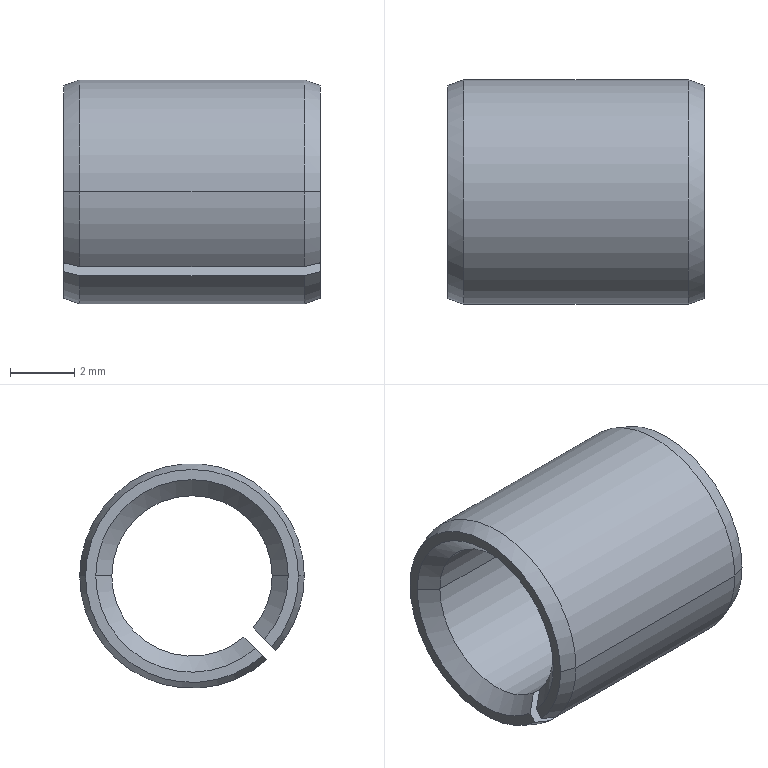Part | NX | 1 solid | 22 faces | box 8 x 7 x 7 mm | volume 141.575 mm3 | cone 12 | cylinder 6 | plane 4 | commonest cylinder face diameters 5 x3 7 x3
STEP:
#1=CARTESIAN_POINT('',(0.5,-2.5,0.));
#2=VERTEX_POINT('',#1);
#3=CARTESIAN_POINT('',(0.,-3.,0.));
#4=VERTEX_POINT('',#3);
#5=CARTESIAN_POINT('',(0.25,-2.75,0.));
#6=DIRECTION('',(-0.7071,-0.7071,0.));
#7=VECTOR('',#6,1000.);
#8=LINE('',#5,#7);
#9=EDGE_CURVE('',#2,#4,#8,.T.);
#10=ORIENTED_EDGE('',*,*,#9,.F.);
#11=CARTESIAN_POINT('',(0.5,-1.904,-1.621));
#12=VERTEX_POINT('',#11);
#13=CARTESIAN_POINT('',(0.5,0.,0.));
#14=DIRECTION('',(-1.,0.,0.));
#15=DIRECTION('',(0.,1.,0.));
#16=AXIS2_PLACEMENT_3D('',#13,#14,#15);
#17=CIRCLE('',#16,2.5);
#18=EDGE_CURVE('',#12,#2,#17,.T.);
#19=ORIENTED_EDGE('',*,*,#18,.F.);
#20=CARTESIAN_POINT('',(0.,-2.258,-1.975));
#21=VERTEX_POINT('',#20);
#22=CARTESIAN_POINT('',(0.5,-1.904,-1.621));
#23=CARTESIAN_POINT('',(0.2728,-2.065,-1.782));
#24=CARTESIAN_POINT('',(0.,-2.258,-1.975));
#25=(BOUNDED_CURVE()B_SPLINE_CURVE(2,(#22,#23,#24),.UNSPECIFIED.,.F.,.F.)B_SPLINE_CURVE_WITH_KNOTS((3,3),(0.,0.7081),.UNSPECIFIED.)CURVE()GEOMETRIC_REPRESENTATION_ITEM()RATIONAL_B_SPLINE_CURVE((1.,1.004,1.))REPRESENTATION_ITEM(''));
#26=EDGE_CURVE('',#12,#21,#25,.T.);
#27=ORIENTED_EDGE('',*,*,#26,.T.);
#28=CARTESIAN_POINT('',(0.,0.,0.));
#29=DIRECTION('',(-1.,0.,0.));
#30=DIRECTION('',(0.,1.,0.));
#31=AXIS2_PLACEMENT_3D('',#28,#29,#30);
#32=CIRCLE('',#31,3.);
#33=EDGE_CURVE('',#21,#4,#32,.T.);
#34=ORIENTED_EDGE('',*,*,#33,.T.);
#35=EDGE_LOOP('',(#10,#19,#27,#34));
#36=FACE_BOUND('',#35,.T.);
#37=CARTESIAN_POINT('',(0.25,0.,0.));
#38=DIRECTION('',(-1.,0.,0.));
#39=DIRECTION('',(0.,1.,0.));
#40=AXIS2_PLACEMENT_3D('',#37,#38,#39);
#41=CONICAL_SURFACE('',#40,2.75,0.7854);
#42=ADVANCED_FACE('',(#36),#41,.F.);
#43=CARTESIAN_POINT('',(8.,-1.975,-2.258));
#44=VERTEX_POINT('',#43);
#45=CARTESIAN_POINT('',(8.,-2.201,-2.483));
#46=VERTEX_POINT('',#45);
#47=CARTESIAN_POINT('',(8.,0.9312,0.6483));
#48=DIRECTION('',(0.,-0.7071,-0.7071));
#49=VECTOR('',#48,1000.);
#50=LINE('',#47,#49);
#51=EDGE_CURVE('',#44,#46,#50,.T.);
#52=ORIENTED_EDGE('',*,*,#51,.T.);
#53=CARTESIAN_POINT('',(8.,3.318,0.));
#54=VERTEX_POINT('',#53);
#55=CARTESIAN_POINT('',(8.,0.,0.));
#56=DIRECTION('',(-1.,0.,0.));
#57=DIRECTION('',(0.,1.,0.));
#58=AXIS2_PLACEMENT_3D('',#55,#56,#57);
#59=CIRCLE('',#58,3.318);
#60=EDGE_CURVE('',#54,#46,#59,.T.);
#61=ORIENTED_EDGE('',*,*,#60,.F.);
#62=CARTESIAN_POINT('',(8.,-3.318,0.));
#63=VERTEX_POINT('',#62);
#64=CARTESIAN_POINT('',(8.,0.,0.));
#65=DIRECTION('',(-1.,0.,0.));
#66=DIRECTION('',(0.,1.,0.));
#67=AXIS2_PLACEMENT_3D('',#64,#65,#66);
#68=CIRCLE('',#67,3.318);
#69=EDGE_CURVE('',#63,#54,#68,.T.);
#70=ORIENTED_EDGE('',*,*,#69,.F.);
#71=CARTESIAN_POINT('',(8.,-2.483,-2.201));
#72=VERTEX_POINT('',#71);
#73=CARTESIAN_POINT('',(8.,0.,0.));
#74=DIRECTION('',(-1.,0.,0.));
#75=DIRECTION('',(0.,1.,0.));
#76=AXIS2_PLACEMENT_3D('',#73,#74,#75);
#77=CIRCLE('',#76,3.318);
#78=EDGE_CURVE('',#72,#63,#77,.T.);
#79=ORIENTED_EDGE('',*,*,#78,.F.);
#80=CARTESIAN_POINT('',(8.,-2.258,-1.975));
#81=VERTEX_POINT('',#80);
#82=CARTESIAN_POINT('',(8.,-1.827,-1.544));
#83=DIRECTION('',(0.,0.7071,0.7071));
#84=VECTOR('',#83,1000.);
#85=LINE('',#82,#84);
#86=EDGE_CURVE('',#72,#81,#85,.T.);
#87=ORIENTED_EDGE('',*,*,#86,.T.);
#88=CARTESIAN_POINT('',(8.,-3.,0.));
#89=VERTEX_POINT('',#88);
#90=CARTESIAN_POINT('',(8.,0.,0.));
#91=DIRECTION('',(-1.,0.,0.));
#92=DIRECTION('',(0.,1.,0.));
#93=AXIS2_PLACEMENT_3D('',#90,#91,#92);
#94=CIRCLE('',#93,3.);
#95=EDGE_CURVE('',#81,#89,#94,.T.);
#96=ORIENTED_EDGE('',*,*,#95,.T.);
#97=CARTESIAN_POINT('',(8.,3.,0.));
#98=VERTEX_POINT('',#97);
#99=CARTESIAN_POINT('',(8.,0.,0.));
#100=DIRECTION('',(-1.,0.,0.));
#101=DIRECTION('',(0.,1.,0.));
#102=AXIS2_PLACEMENT_3D('',#99,#100,#101);
#103=CIRCLE('',#102,3.);
#104=EDGE_CURVE('',#89,#98,#103,.T.);
#105=ORIENTED_EDGE('',*,*,#104,.T.);
#106=CARTESIAN_POINT('',(8.,0.,0.));
#107=DIRECTION('',(-1.,0.,0.));
#108=DIRECTION('',(0.,1.,0.));
#109=AXIS2_PLACEMENT_3D('',#106,#107,#108);
#110=CIRCLE('',#109,3.);
#111=EDGE_CURVE('',#98,#44,#110,.T.);
#112=ORIENTED_EDGE('',*,*,#111,.T.);
#113=EDGE_LOOP('',(#52,#61,#70,#79,#87,#96,#105,#112));
#114=FACE_BOUND('',#113,.T.);
#115=CARTESIAN_POINT('',(8.,3.159,0.));
#116=DIRECTION('',(1.,0.,0.));
#117=DIRECTION('',(0.,0.,1.));
#118=AXIS2_PLACEMENT_3D('',#115,#116,#117);
#119=PLANE('',#118);
#120=ADVANCED_FACE('',(#114),#119,.T.);
#121=CARTESIAN_POINT('',(0.5,-3.5,0.));
#122=VERTEX_POINT('',#121);
#123=CARTESIAN_POINT('',(7.5,-3.5,0.));
#124=VERTEX_POINT('',#123);
#125=CARTESIAN_POINT('',(4.,-3.5,0.));
#126=DIRECTION('',(1.,0.,0.));
#127=VECTOR('',#126,1000.);
#128=LINE('',#125,#127);
#129=EDGE_CURVE('',#122,#124,#128,.T.);
#130=ORIENTED_EDGE('',*,*,#129,.F.);
#131=CARTESIAN_POINT('',(0.5,-2.612,-2.329));
#132=VERTEX_POINT('',#131);
#133=CARTESIAN_POINT('',(0.5,0.,0.));
#134=DIRECTION('',(-1.,0.,0.));
#135=DIRECTION('',(0.,1.,0.));
#136=AXIS2_PLACEMENT_3D('',#133,#134,#135);
#137=CIRCLE('',#136,3.5);
#138=EDGE_CURVE('',#132,#122,#137,.T.);
#139=ORIENTED_EDGE('',*,*,#138,.F.);
#140=CARTESIAN_POINT('',(7.5,-2.612,-2.329));
#141=VERTEX_POINT('',#140);
#142=CARTESIAN_POINT('',(4.,-2.612,-2.329));
#143=DIRECTION('',(1.,0.,0.));
#144=VECTOR('',#143,1000.);
#145=LINE('',#142,#144);
#146=EDGE_CURVE('',#132,#141,#145,.T.);
#147=ORIENTED_EDGE('',*,*,#146,.T.);
#148=CARTESIAN_POINT('',(7.5,0.,0.));
#149=DIRECTION('',(-1.,0.,0.));
#150=DIRECTION('',(0.,1.,0.));
#151=AXIS2_PLACEMENT_3D('',#148,#149,#150);
#152=CIRCLE('',#151,3.5);
#153=EDGE_CURVE('',#141,#124,#152,.T.);
#154=ORIENTED_EDGE('',*,*,#153,.T.);
#155=EDGE_LOOP('',(#130,#139,#147,#154));
#156=FACE_BOUND('',#155,.T.);
#157=CARTESIAN_POINT('',(4.,0.,0.));
#158=DIRECTION('',(1.,0.,0.));
#159=DIRECTION('',(0.,1.,0.));
#160=AXIS2_PLACEMENT_3D('',#157,#158,#159);
#161=CYLINDRICAL_SURFACE('',#160,3.5);
#162=ADVANCED_FACE('',(#156),#161,.T.);
#163=CARTESIAN_POINT('',(0.,-2.201,-2.483));
#164=VERTEX_POINT('',#163);
#165=CARTESIAN_POINT('',(0.,-1.975,-2.258));
#166=VERTEX_POINT('',#165);
#167=CARTESIAN_POINT('',(0.,0.9312,0.6483));
#168=DIRECTION('',(0.,0.7071,0.7071));
#169=VECTOR('',#168,1000.);
#170=LINE('',#167,#169);
#171=EDGE_CURVE('',#164,#166,#170,.T.);
#172=ORIENTED_EDGE('',*,*,#171,.T.);
#173=CARTESIAN_POINT('',(0.,3.,0.));
#174=VERTEX_POINT('',#173);
#175=CARTESIAN_POINT('',(0.,0.,0.));
#176=DIRECTION('',(-1.,0.,0.));
#177=DIRECTION('',(0.,1.,0.));
#178=AXIS2_PLACEMENT_3D('',#175,#176,#177);
#179=CIRCLE('',#178,3.);
#180=EDGE_CURVE('',#174,#166,#179,.T.);
#181=ORIENTED_EDGE('',*,*,#180,.F.);
#182=CARTESIAN_POINT('',(0.,0.,0.));
#183=DIRECTION('',(-1.,0.,0.));
#184=DIRECTION('',(0.,1.,0.));
#185=AXIS2_PLACEMENT_3D('',#182,#183,#184);
#186=CIRCLE('',#185,3.);
#187=EDGE_CURVE('',#4,#174,#186,.T.);
#188=ORIENTED_EDGE('',*,*,#187,.F.);
#189=ORIENTED_EDGE('',*,*,#33,.F.);
#190=CARTESIAN_POINT('',(0.,-2.483,-2.201));
#191=VERTEX_POINT('',#190);
#192=CARTESIAN_POINT('',(0.,-1.827,-1.544));
#193=DIRECTION('',(0.,-0.7071,-0.7071));
#194=VECTOR('',#193,1000.);
#195=LINE('',#192,#194);
#196=EDGE_CURVE('',#21,#191,#195,.T.);
#197=ORIENTED_EDGE('',*,*,#196,.T.);
#198=CARTESIAN_POINT('',(0.,-3.318,0.));
#199=VERTEX_POINT('',#198);
#200=CARTESIAN_POINT('',(0.,0.,0.));
#201=DIRECTION('',(-1.,0.,0.));
#202=DIRECTION('',(0.,1.,0.));
#203=AXIS2_PLACEMENT_3D('',#200,#201,#202);
#204=CIRCLE('',#203,3.318);
#205=EDGE_CURVE('',#191,#199,#204,.T.);
#206=ORIENTED_EDGE('',*,*,#205,.T.);
#207=CARTESIAN_POINT('',(0.,3.318,0.));
#208=VERTEX_POINT('',#207);
#209=CARTESIAN_POINT('',(0.,0.,0.));
#210=DIRECTION('',(-1.,0.,0.));
#211=DIRECTION('',(0.,1.,0.));
#212=AXIS2_PLACEMENT_3D('',#209,#210,#211);
#213=CIRCLE('',#212,3.318);
#214=EDGE_CURVE('',#199,#208,#213,.T.);
#215=ORIENTED_EDGE('',*,*,#214,.T.);
#216=CARTESIAN_POINT('',(0.,0.,0.));
#217=DIRECTION('',(-1.,0.,0.));
#218=DIRECTION('',(0.,1.,0.));
#219=AXIS2_PLACEMENT_3D('',#216,#217,#218);
#220=CIRCLE('',#219,3.318);
#221=EDGE_CURVE('',#208,#164,#220,.T.);
#222=ORIENTED_EDGE('',*,*,#221,.T.);
#223=EDGE_LOOP('',(#172,#181,#188,#189,#197,#206,#215,#222));
#224=FACE_BOUND('',#223,.T.);
#225=CARTESIAN_POINT('',(0.,3.159,0.));
#226=DIRECTION('',(-1.,0.,0.));
#227=DIRECTION('',(0.,0.,1.));
#228=AXIS2_PLACEMENT_3D('',#225,#226,#227);
#229=PLANE('',#228);
#230=ADVANCED_FACE('',(#224),#229,.T.);
#231=CARTESIAN_POINT('',(0.,-2.483,-2.201));
#232=CARTESIAN_POINT('',(0.2433,-2.546,-2.263));
#233=CARTESIAN_POINT('',(0.5,-2.612,-2.329));
#234=(BOUNDED_CURVE()B_SPLINE_CURVE(2,(#231,#232,#233),.UNSPECIFIED.,.F.,.F.)B_SPLINE_CURVE_WITH_KNOTS((3,3),(0.,0.5322),.UNSPECIFIED.)CURVE()GEOMETRIC_REPRESENTATION_ITEM()RATIONAL_B_SPLINE_CURVE((1.,1.,1.))REPRESENTATION_ITEM(''));
#235=EDGE_CURVE('',#191,#132,#234,.T.);
#236=ORIENTED_EDGE('',*,*,#235,.F.);
#237=ORIENTED_EDGE('',*,*,#196,.F.);
#238=ORIENTED_EDGE('',*,*,#26,.F.);
#239=CARTESIAN_POINT('',(7.5,-1.904,-1.621));
#240=VERTEX_POINT('',#239);
#241=CARTESIAN_POINT('',(4.,-1.904,-1.621));
#242=DIRECTION('',(-1.,0.,0.));
#243=VECTOR('',#242,1000.);
#244=LINE('',#241,#243);
#245=EDGE_CURVE('',#240,#12,#244,.T.);
#246=ORIENTED_EDGE('',*,*,#245,.F.);
#247=CARTESIAN_POINT('',(8.,-2.258,-1.975));
#248=CARTESIAN_POINT('',(7.727,-2.065,-1.782));
#249=CARTESIAN_POINT('',(7.5,-1.904,-1.621));
#250=(BOUNDED_CURVE()B_SPLINE_CURVE(2,(#247,#248,#249),.UNSPECIFIED.,.F.,.F.)B_SPLINE_CURVE_WITH_KNOTS((3,3),(0.,0.7081),.UNSPECIFIED.)CURVE()GEOMETRIC_REPRESENTATION_ITEM()RATIONAL_B_SPLINE_CURVE((1.,1.004,1.))REPRESENTATION_ITEM(''));
#251=EDGE_CURVE('',#81,#240,#250,.T.);
#252=ORIENTED_EDGE('',*,*,#251,.F.);
#253=ORIENTED_EDGE('',*,*,#86,.F.);
#254=CARTESIAN_POINT('',(7.5,-2.612,-2.329));
#255=CARTESIAN_POINT('',(7.757,-2.546,-2.263));
#256=CARTESIAN_POINT('',(8.,-2.483,-2.201));
#257=(BOUNDED_CURVE()B_SPLINE_CURVE(2,(#254,#255,#256),.UNSPECIFIED.,.F.,.F.)B_SPLINE_CURVE_WITH_KNOTS((3,3),(0.,0.5322),.UNSPECIFIED.)CURVE()GEOMETRIC_REPRESENTATION_ITEM()RATIONAL_B_SPLINE_CURVE((1.,1.,1.))REPRESENTATION_ITEM(''));
#258=EDGE_CURVE('',#141,#72,#257,.T.);
#259=ORIENTED_EDGE('',*,*,#258,.F.);
#260=ORIENTED_EDGE('',*,*,#146,.F.);
#261=EDGE_LOOP('',(#236,#237,#238,#246,#252,#253,#259,#260));
#262=FACE_BOUND('',#261,.T.);
#263=CARTESIAN_POINT('',(0.,-5.091,-4.808));
#264=DIRECTION('',(0.,-0.7071,0.7071));
#265=DIRECTION('',(-1.,0.,0.));
#266=AXIS2_PLACEMENT_3D('',#263,#264,#265);
#267=PLANE('',#266);
#268=ADVANCED_FACE('',(#262),#267,.F.);
#269=CARTESIAN_POINT('',(7.5,3.5,0.));
#270=VERTEX_POINT('',#269);
#271=CARTESIAN_POINT('',(7.75,3.409,0.));
#272=DIRECTION('',(-0.9397,0.342,0.));
#273=VECTOR('',#272,1000.);
#274=LINE('',#271,#273);
#275=EDGE_CURVE('',#54,#270,#274,.T.);
#276=ORIENTED_EDGE('',*,*,#275,.F.);
#277=ORIENTED_EDGE('',*,*,#60,.T.);
#278=CARTESIAN_POINT('',(7.5,-2.329,-2.612));
#279=VERTEX_POINT('',#278);
#280=CARTESIAN_POINT('',(8.,-2.201,-2.483));
#281=CARTESIAN_POINT('',(7.757,-2.263,-2.546));
#282=CARTESIAN_POINT('',(7.5,-2.329,-2.612));
#283=(BOUNDED_CURVE()B_SPLINE_CURVE(2,(#280,#281,#282),.UNSPECIFIED.,.F.,.F.)B_SPLINE_CURVE_WITH_KNOTS((3,3),(0.,0.5322),.UNSPECIFIED.)CURVE()GEOMETRIC_REPRESENTATION_ITEM()RATIONAL_B_SPLINE_CURVE((1.,1.,1.))REPRESENTATION_ITEM(''));
#284=EDGE_CURVE('',#46,#279,#283,.T.);
#285=ORIENTED_EDGE('',*,*,#284,.T.);
#286=CARTESIAN_POINT('',(7.5,0.,0.));
#287=DIRECTION('',(-1.,0.,0.));
#288=DIRECTION('',(0.,1.,0.));
#289=AXIS2_PLACEMENT_3D('',#286,#287,#288);
#290=CIRCLE('',#289,3.5);
#291=EDGE_CURVE('',#270,#279,#290,.T.);
#292=ORIENTED_EDGE('',*,*,#291,.F.);
#293=EDGE_LOOP('',(#276,#277,#285,#292));
#294=FACE_BOUND('',#293,.T.);
#295=CARTESIAN_POINT('',(7.75,0.,0.));
#296=DIRECTION('',(-1.,0.,0.));
#297=DIRECTION('',(0.,1.,0.));
#298=AXIS2_PLACEMENT_3D('',#295,#296,#297);
#299=CONICAL_SURFACE('',#298,3.409,0.3491);
#300=ADVANCED_FACE('',(#294),#299,.T.);
#301=CARTESIAN_POINT('',(0.5,2.5,0.));
#302=VERTEX_POINT('',#301);
#303=CARTESIAN_POINT('',(7.5,2.5,0.));
#304=VERTEX_POINT('',#303);
#305=CARTESIAN_POINT('',(4.,2.5,0.));
#306=DIRECTION('',(1.,0.,0.));
#307=VECTOR('',#306,1000.);
#308=LINE('',#305,#307);
#309=EDGE_CURVE('',#302,#304,#308,.T.);
#310=ORIENTED_EDGE('',*,*,#309,.F.);
#311=CARTESIAN_POINT('',(0.5,-1.621,-1.904));
#312=VERTEX_POINT('',#311);
#313=CARTESIAN_POINT('',(0.5,0.,0.));
#314=DIRECTION('',(-1.,0.,0.));
#315=DIRECTION('',(0.,1.,0.));
#316=AXIS2_PLACEMENT_3D('',#313,#314,#315);
#317=CIRCLE('',#316,2.5);
#318=EDGE_CURVE('',#302,#312,#317,.T.);
#319=ORIENTED_EDGE('',*,*,#318,.T.);
#320=CARTESIAN_POINT('',(7.5,-1.621,-1.904));
#321=VERTEX_POINT('',#320);
#322=CARTESIAN_POINT('',(4.,-1.621,-1.904));
#323=DIRECTION('',(1.,0.,0.));
#324=VECTOR('',#323,1000.);
#325=LINE('',#322,#324);
#326=EDGE_CURVE('',#312,#321,#325,.T.);
#327=ORIENTED_EDGE('',*,*,#326,.T.);
#328=CARTESIAN_POINT('',(7.5,0.,0.));
#329=DIRECTION('',(-1.,0.,0.));
#330=DIRECTION('',(0.,1.,0.));
#331=AXIS2_PLACEMENT_3D('',#328,#329,#330);
#332=CIRCLE('',#331,2.5);
#333=EDGE_CURVE('',#304,#321,#332,.T.);
#334=ORIENTED_EDGE('',*,*,#333,.F.);
#335=EDGE_LOOP('',(#310,#319,#327,#334));
#336=FACE_BOUND('',#335,.T.);
#337=CARTESIAN_POINT('',(4.,0.,0.));
#338=DIRECTION('',(1.,0.,0.));
#339=DIRECTION('',(0.,1.,0.));
#340=AXIS2_PLACEMENT_3D('',#337,#338,#339);
#341=CYLINDRICAL_SURFACE('',#340,2.5);
#342=ADVANCED_FACE('',(#336),#341,.F.);
#343=CARTESIAN_POINT('',(0.25,-3.409,0.));
#344=DIRECTION('',(0.9397,-0.342,0.));
#345=VECTOR('',#344,1000.);
#346=LINE('',#343,#345);
#347=EDGE_CURVE('',#199,#122,#346,.T.);
#348=ORIENTED_EDGE('',*,*,#347,.F.);
#349=ORIENTED_EDGE('',*,*,#205,.F.);
#350=ORIENTED_EDGE('',*,*,#235,.T.);
#351=ORIENTED_EDGE('',*,*,#138,.T.);
#352=EDGE_LOOP('',(#348,#349,#350,#351));
#353=FACE_BOUND('',#352,.T.);
#354=CARTESIAN_POINT('',(0.25,0.,0.));
#355=DIRECTION('',(1.,0.,0.));
#356=DIRECTION('',(0.,-1.,0.));
#357=AXIS2_PLACEMENT_3D('',#354,#355,#356);
#358=CONICAL_SURFACE('',#357,3.409,0.3491);
#359=ADVANCED_FACE('',(#353),#358,.T.);
#360=CARTESIAN_POINT('',(7.75,2.75,0.));
#361=DIRECTION('',(0.7071,0.7071,0.));
#362=VECTOR('',#361,1000.);
#363=LINE('',#360,#362);
#364=EDGE_CURVE('',#304,#98,#363,.T.);
#365=ORIENTED_EDGE('',*,*,#364,.F.);
#366=ORIENTED_EDGE('',*,*,#333,.T.);
#367=CARTESIAN_POINT('',(7.5,-1.621,-1.904));
#368=CARTESIAN_POINT('',(7.727,-1.782,-2.065));
#369=CARTESIAN_POINT('',(8.,-1.975,-2.258));
#370=(BOUNDED_CURVE()B_SPLINE_CURVE(2,(#367,#368,#369),.UNSPECIFIED.,.F.,.F.)B_SPLINE_CURVE_WITH_KNOTS((3,3),(0.,0.7081),.UNSPECIFIED.)CURVE()GEOMETRIC_REPRESENTATION_ITEM()RATIONAL_B_SPLINE_CURVE((1.,1.004,1.))REPRESENTATION_ITEM(''));
#371=EDGE_CURVE('',#321,#44,#370,.T.);
#372=ORIENTED_EDGE('',*,*,#371,.T.);
#373=ORIENTED_EDGE('',*,*,#111,.F.);
#374=EDGE_LOOP('',(#365,#366,#372,#373));
#375=FACE_BOUND('',#374,.T.);
#376=CARTESIAN_POINT('',(7.75,0.,0.));
#377=DIRECTION('',(1.,0.,0.));
#378=DIRECTION('',(0.,-1.,0.));
#379=AXIS2_PLACEMENT_3D('',#376,#377,#378);
#380=CONICAL_SURFACE('',#379,2.75,0.7854);
#381=ADVANCED_FACE('',(#375),#380,.F.);
#382=CARTESIAN_POINT('',(0.5,-2.329,-2.612));
#383=VERTEX_POINT('',#382);
#384=CARTESIAN_POINT('',(0.5,-2.329,-2.612));
#385=CARTESIAN_POINT('',(0.2433,-2.263,-2.546));
#386=CARTESIAN_POINT('',(0.,-2.201,-2.483));
#387=(BOUNDED_CURVE()B_SPLINE_CURVE(2,(#384,#385,#386),.UNSPECIFIED.,.F.,.F.)B_SPLINE_CURVE_WITH_KNOTS((3,3),(0.,0.5322),.UNSPECIFIED.)CURVE()GEOMETRIC_REPRESENTATION_ITEM()RATIONAL_B_SPLINE_CURVE((1.,1.,1.))REPRESENTATION_ITEM(''));
#388=EDGE_CURVE('',#383,#164,#387,.T.);
#389=ORIENTED_EDGE('',*,*,#388,.F.);
#390=CARTESIAN_POINT('',(4.,-2.329,-2.612));
#391=DIRECTION('',(-1.,0.,0.));
#392=VECTOR('',#391,1000.);
#393=LINE('',#390,#392);
#394=EDGE_CURVE('',#279,#383,#393,.T.);
#395=ORIENTED_EDGE('',*,*,#394,.F.);
#396=ORIENTED_EDGE('',*,*,#284,.F.);
#397=ORIENTED_EDGE('',*,*,#51,.F.);
#398=ORIENTED_EDGE('',*,*,#371,.F.);
#399=ORIENTED_EDGE('',*,*,#326,.F.);
#400=CARTESIAN_POINT('',(0.,-1.975,-2.258));
#401=CARTESIAN_POINT('',(0.2728,-1.782,-2.065));
#402=CARTESIAN_POINT('',(0.5,-1.621,-1.904));
#403=(BOUNDED_CURVE()B_SPLINE_CURVE(2,(#400,#401,#402),.UNSPECIFIED.,.F.,.F.)B_SPLINE_CURVE_WITH_KNOTS((3,3),(0.,0.7081),.UNSPECIFIED.)CURVE()GEOMETRIC_REPRESENTATION_ITEM()RATIONAL_B_SPLINE_CURVE((1.,1.004,1.))REPRESENTATION_ITEM(''));
#404=EDGE_CURVE('',#166,#312,#403,.T.);
#405=ORIENTED_EDGE('',*,*,#404,.F.);
#406=ORIENTED_EDGE('',*,*,#171,.F.);
#407=EDGE_LOOP('',(#389,#395,#396,#397,#398,#399,#405,#406));
#408=FACE_BOUND('',#407,.T.);
#409=CARTESIAN_POINT('',(0.,0.1414,-0.1414));
#410=DIRECTION('',(0.,0.7071,-0.7071));
#411=DIRECTION('',(-1.,0.,0.));
#412=AXIS2_PLACEMENT_3D('',#409,#410,#411);
#413=PLANE('',#412);
#414=ADVANCED_FACE('',(#408),#413,.F.);
#415=CARTESIAN_POINT('',(7.5,-2.5,0.));
#416=VERTEX_POINT('',#415);
#417=CARTESIAN_POINT('',(7.5,0.,0.));
#418=DIRECTION('',(-1.,0.,0.));
#419=DIRECTION('',(0.,1.,0.));
#420=AXIS2_PLACEMENT_3D('',#417,#418,#419);
#421=CIRCLE('',#420,2.5);
#422=EDGE_CURVE('',#240,#416,#421,.T.);
#423=ORIENTED_EDGE('',*,*,#422,.T.);
#424=CARTESIAN_POINT('',(7.75,-2.75,0.));
#425=DIRECTION('',(0.7071,-0.7071,0.));
#426=VECTOR('',#425,1000.);
#427=LINE('',#424,#426);
#428=EDGE_CURVE('',#416,#89,#427,.T.);
#429=ORIENTED_EDGE('',*,*,#428,.T.);
#430=ORIENTED_EDGE('',*,*,#95,.F.);
#431=ORIENTED_EDGE('',*,*,#251,.T.);
#432=EDGE_LOOP('',(#423,#429,#430,#431));
#433=FACE_BOUND('',#432,.T.);
#434=CARTESIAN_POINT('',(7.75,0.,0.));
#435=DIRECTION('',(1.,0.,0.));
#436=DIRECTION('',(0.,-1.,0.));
#437=AXIS2_PLACEMENT_3D('',#434,#435,#436);
#438=CONICAL_SURFACE('',#437,2.75,0.7854);
#439=ADVANCED_FACE('',(#433),#438,.F.);
#440=CARTESIAN_POINT('',(7.5,0.,0.));
#441=DIRECTION('',(-1.,0.,0.));
#442=DIRECTION('',(0.,1.,0.));
#443=AXIS2_PLACEMENT_3D('',#440,#441,#442);
#444=CIRCLE('',#443,2.5);
#445=EDGE_CURVE('',#416,#304,#444,.T.);
#446=ORIENTED_EDGE('',*,*,#445,.T.);
#447=ORIENTED_EDGE('',*,*,#364,.T.);
#448=ORIENTED_EDGE('',*,*,#104,.F.);
#449=ORIENTED_EDGE('',*,*,#428,.F.);
#450=EDGE_LOOP('',(#446,#447,#448,#449));
#451=FACE_BOUND('',#450,.T.);
#452=CARTESIAN_POINT('',(7.75,0.,0.));
#453=DIRECTION('',(1.,0.,0.));
#454=DIRECTION('',(0.,-1.,0.));
#455=AXIS2_PLACEMENT_3D('',#452,#453,#454);
#456=CONICAL_SURFACE('',#455,2.75,0.7854);
#457=ADVANCED_FACE('',(#451),#456,.F.);
#458=CARTESIAN_POINT('',(0.5,3.5,0.));
#459=VERTEX_POINT('',#458);
#460=CARTESIAN_POINT('',(0.25,3.409,0.));
#461=DIRECTION('',(0.9397,0.342,0.));
#462=VECTOR('',#461,1000.);
#463=LINE('',#460,#462);
#464=EDGE_CURVE('',#208,#459,#463,.T.);
#465=ORIENTED_EDGE('',*,*,#464,.F.);
#466=ORIENTED_EDGE('',*,*,#214,.F.);
#467=ORIENTED_EDGE('',*,*,#347,.T.);
#468=CARTESIAN_POINT('',(0.5,0.,0.));
#469=DIRECTION('',(-1.,0.,0.));
#470=DIRECTION('',(0.,1.,0.));
#471=AXIS2_PLACEMENT_3D('',#468,#469,#470);
#472=CIRCLE('',#471,3.5);
#473=EDGE_CURVE('',#122,#459,#472,.T.);
#474=ORIENTED_EDGE('',*,*,#473,.T.);
#475=EDGE_LOOP('',(#465,#466,#467,#474));
#476=FACE_BOUND('',#475,.T.);
#477=CARTESIAN_POINT('',(0.25,0.,0.));
#478=DIRECTION('',(1.,0.,0.));
#479=DIRECTION('',(0.,-1.,0.));
#480=AXIS2_PLACEMENT_3D('',#477,#478,#479);
#481=CONICAL_SURFACE('',#480,3.409,0.3491);
#482=ADVANCED_FACE('',(#476),#481,.T.);
#483=ORIENTED_EDGE('',*,*,#221,.F.);
#484=ORIENTED_EDGE('',*,*,#464,.T.);
#485=CARTESIAN_POINT('',(0.5,0.,0.));
#486=DIRECTION('',(-1.,0.,0.));
#487=DIRECTION('',(0.,1.,0.));
#488=AXIS2_PLACEMENT_3D('',#485,#486,#487);
#489=CIRCLE('',#488,3.5);
#490=EDGE_CURVE('',#459,#383,#489,.T.);
#491=ORIENTED_EDGE('',*,*,#490,.T.);
#492=ORIENTED_EDGE('',*,*,#388,.T.);
#493=EDGE_LOOP('',(#483,#484,#491,#492));
#494=FACE_BOUND('',#493,.T.);
#495=CARTESIAN_POINT('',(0.25,0.,0.));
#496=DIRECTION('',(1.,0.,0.));
#497=DIRECTION('',(0.,-1.,0.));
#498=AXIS2_PLACEMENT_3D('',#495,#496,#497);
#499=CONICAL_SURFACE('',#498,3.409,0.3491);
#500=ADVANCED_FACE('',(#494),#499,.T.);
#501=CARTESIAN_POINT('',(4.,-2.5,0.));
#502=DIRECTION('',(1.,0.,0.));
#503=VECTOR('',#502,1000.);
#504=LINE('',#501,#503);
#505=EDGE_CURVE('',#2,#416,#504,.T.);
#506=ORIENTED_EDGE('',*,*,#505,.F.);
#507=CARTESIAN_POINT('',(0.5,0.,0.));
#508=DIRECTION('',(-1.,0.,0.));
#509=DIRECTION('',(0.,1.,0.));
#510=AXIS2_PLACEMENT_3D('',#507,#508,#509);
#511=CIRCLE('',#510,2.5);
#512=EDGE_CURVE('',#2,#302,#511,.T.);
#513=ORIENTED_EDGE('',*,*,#512,.T.);
#514=ORIENTED_EDGE('',*,*,#309,.T.);
#515=ORIENTED_EDGE('',*,*,#445,.F.);
#516=EDGE_LOOP('',(#506,#513,#514,#515));
#517=FACE_BOUND('',#516,.T.);
#518=CARTESIAN_POINT('',(4.,0.,0.));
#519=DIRECTION('',(1.,0.,0.));
#520=DIRECTION('',(0.,1.,0.));
#521=AXIS2_PLACEMENT_3D('',#518,#519,#520);
#522=CYLINDRICAL_SURFACE('',#521,2.5);
#523=ADVANCED_FACE('',(#517),#522,.F.);
#524=ORIENTED_EDGE('',*,*,#18,.T.);
#525=ORIENTED_EDGE('',*,*,#505,.T.);
#526=ORIENTED_EDGE('',*,*,#422,.F.);
#527=ORIENTED_EDGE('',*,*,#245,.T.);
#528=EDGE_LOOP('',(#524,#525,#526,#527));
#529=FACE_BOUND('',#528,.T.);
#530=CARTESIAN_POINT('',(4.,0.,0.));
#531=DIRECTION('',(1.,0.,0.));
#532=DIRECTION('',(0.,1.,0.));
#533=AXIS2_PLACEMENT_3D('',#530,#531,#532);
#534=CYLINDRICAL_SURFACE('',#533,2.5);
#535=ADVANCED_FACE('',(#529),#534,.F.);
#536=CARTESIAN_POINT('',(7.75,-3.409,0.));
#537=DIRECTION('',(-0.9397,-0.342,0.));
#538=VECTOR('',#537,1000.);
#539=LINE('',#536,#538);
#540=EDGE_CURVE('',#63,#124,#539,.T.);
#541=ORIENTED_EDGE('',*,*,#540,.F.);
#542=ORIENTED_EDGE('',*,*,#69,.T.);
#543=ORIENTED_EDGE('',*,*,#275,.T.);
#544=CARTESIAN_POINT('',(7.5,0.,0.));
#545=DIRECTION('',(-1.,0.,0.));
#546=DIRECTION('',(0.,1.,0.));
#547=AXIS2_PLACEMENT_3D('',#544,#545,#546);
#548=CIRCLE('',#547,3.5);
#549=EDGE_CURVE('',#124,#270,#548,.T.);
#550=ORIENTED_EDGE('',*,*,#549,.F.);
#551=EDGE_LOOP('',(#541,#542,#543,#550));
#552=FACE_BOUND('',#551,.T.);
#553=CARTESIAN_POINT('',(7.75,0.,0.));
#554=DIRECTION('',(-1.,0.,0.));
#555=DIRECTION('',(0.,1.,0.));
#556=AXIS2_PLACEMENT_3D('',#553,#554,#555);
#557=CONICAL_SURFACE('',#556,3.409,0.3491);
#558=ADVANCED_FACE('',(#552),#557,.T.);
#559=ORIENTED_EDGE('',*,*,#78,.T.);
#560=ORIENTED_EDGE('',*,*,#540,.T.);
#561=ORIENTED_EDGE('',*,*,#153,.F.);
#562=ORIENTED_EDGE('',*,*,#258,.T.);
#563=EDGE_LOOP('',(#559,#560,#561,#562));
#564=FACE_BOUND('',#563,.T.);
#565=CARTESIAN_POINT('',(7.75,0.,0.));
#566=DIRECTION('',(-1.,0.,0.));
#567=DIRECTION('',(0.,1.,0.));
#568=AXIS2_PLACEMENT_3D('',#565,#566,#567);
#569=CONICAL_SURFACE('',#568,3.409,0.3491);
#570=ADVANCED_FACE('',(#564),#569,.T.);
#571=ORIENTED_EDGE('',*,*,#490,.F.);
#572=CARTESIAN_POINT('',(4.,3.5,0.));
#573=DIRECTION('',(1.,0.,0.));
#574=VECTOR('',#573,1000.);
#575=LINE('',#572,#574);
#576=EDGE_CURVE('',#459,#270,#575,.T.);
#577=ORIENTED_EDGE('',*,*,#576,.T.);
#578=ORIENTED_EDGE('',*,*,#291,.T.);
#579=ORIENTED_EDGE('',*,*,#394,.T.);
#580=EDGE_LOOP('',(#571,#577,#578,#579));
#581=FACE_BOUND('',#580,.T.);
#582=CARTESIAN_POINT('',(4.,0.,0.));
#583=DIRECTION('',(1.,0.,0.));
#584=DIRECTION('',(0.,1.,0.));
#585=AXIS2_PLACEMENT_3D('',#582,#583,#584);
#586=CYLINDRICAL_SURFACE('',#585,3.5);
#587=ADVANCED_FACE('',(#581),#586,.T.);
#588=ORIENTED_EDGE('',*,*,#473,.F.);
#589=ORIENTED_EDGE('',*,*,#129,.T.);
#590=ORIENTED_EDGE('',*,*,#549,.T.);
#591=ORIENTED_EDGE('',*,*,#576,.F.);
#592=EDGE_LOOP('',(#588,#589,#590,#591));
#593=FACE_BOUND('',#592,.T.);
#594=CARTESIAN_POINT('',(4.,0.,0.));
#595=DIRECTION('',(1.,0.,0.));
#596=DIRECTION('',(0.,1.,0.));
#597=AXIS2_PLACEMENT_3D('',#594,#595,#596);
#598=CYLINDRICAL_SURFACE('',#597,3.5);
#599=ADVANCED_FACE('',(#593),#598,.T.);
#600=ORIENTED_EDGE('',*,*,#318,.F.);
#601=CARTESIAN_POINT('',(0.25,2.75,0.));
#602=DIRECTION('',(-0.7071,0.7071,0.));
#603=VECTOR('',#602,1000.);
#604=LINE('',#601,#603);
#605=EDGE_CURVE('',#302,#174,#604,.T.);
#606=ORIENTED_EDGE('',*,*,#605,.T.);
#607=ORIENTED_EDGE('',*,*,#180,.T.);
#608=ORIENTED_EDGE('',*,*,#404,.T.);
#609=EDGE_LOOP('',(#600,#606,#607,#608));
#610=FACE_BOUND('',#609,.T.);
#611=CARTESIAN_POINT('',(0.25,0.,0.));
#612=DIRECTION('',(-1.,0.,0.));
#613=DIRECTION('',(0.,1.,0.));
#614=AXIS2_PLACEMENT_3D('',#611,#612,#613);
#615=CONICAL_SURFACE('',#614,2.75,0.7854);
#616=ADVANCED_FACE('',(#610),#615,.F.);
#617=ORIENTED_EDGE('',*,*,#512,.F.);
#618=ORIENTED_EDGE('',*,*,#9,.T.);
#619=ORIENTED_EDGE('',*,*,#187,.T.);
#620=ORIENTED_EDGE('',*,*,#605,.F.);
#621=EDGE_LOOP('',(#617,#618,#619,#620));
#622=FACE_BOUND('',#621,.T.);
#623=CARTESIAN_POINT('',(0.25,0.,0.));
#624=DIRECTION('',(-1.,0.,0.));
#625=DIRECTION('',(0.,1.,0.));
#626=AXIS2_PLACEMENT_3D('',#623,#624,#625);
#627=CONICAL_SURFACE('',#626,2.75,0.7854);
#628=ADVANCED_FACE('',(#622),#627,.F.);
#629=CLOSED_SHELL('',(#42,#120,#162,#230,#268,#300,#342,#359,#381,#414,#439,#457,#482,#500,#523,#535,#558,#570,#587,#599,#616,#628));
#630=MANIFOLD_SOLID_BREP('',#629);
#631=(LENGTH_UNIT()NAMED_UNIT(*)SI_UNIT(.MILLI.,.METRE.));
#632=UNCERTAINTY_MEASURE_WITH_UNIT(LENGTH_MEASURE(0.00001),#631,'','');
#633=(NAMED_UNIT(*)PLANE_ANGLE_UNIT()SI_UNIT($,.RADIAN.));
#634=(NAMED_UNIT(*)SI_UNIT($,.STERADIAN.)SOLID_ANGLE_UNIT());
#635=(GEOMETRIC_REPRESENTATION_CONTEXT(3)GLOBAL_UNCERTAINTY_ASSIGNED_CONTEXT((#632))GLOBAL_UNIT_ASSIGNED_CONTEXT((#631,#633,#634))REPRESENTATION_CONTEXT('',''));
#636=ADVANCED_BREP_SHAPE_REPRESENTATION('',(#630),#635);